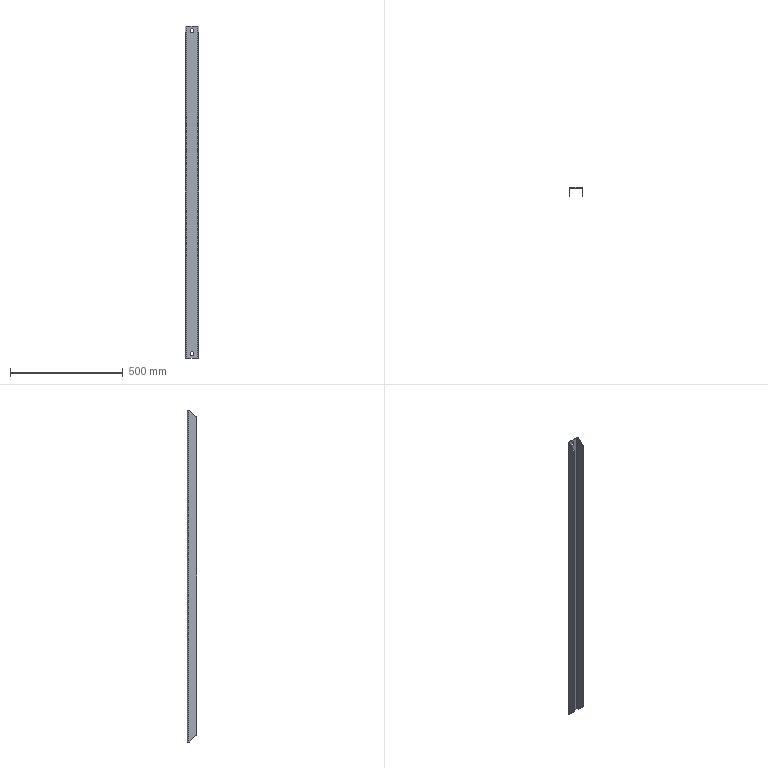Part | STEP file | VD-SYL0380DJ1006_1-2_VD-SYL0380 | 1 solid | 32 faces | box 60 x 40 x 1470 mm | volume 567408 mm3 | plane 18 | cylinder 14 | commonest cylinder face diameters 10 x6 20 x4 6 x2 12 x2
STEP:
#1=CARTESIAN_POINT('',(-5.,20.,-720.));
#2=VERTEX_POINT('',#1);
#3=CARTESIAN_POINT('',(0.,20.,-725.));
#4=VERTEX_POINT('',#3);
#5=CARTESIAN_POINT('',(0.,20.,-720.));
#6=DIRECTION('',(0.,-1.,0.));
#7=DIRECTION('',(-1.,0.,0.));
#8=AXIS2_PLACEMENT_3D('',#5,#6,#7);
#9=CIRCLE('',#8,5.);
#10=EDGE_CURVE('',#2,#4,#9,.T.);
#11=ORIENTED_EDGE('',*,*,#10,.F.);
#12=CARTESIAN_POINT('',(-5.,17.,-720.));
#13=VERTEX_POINT('',#12);
#14=CARTESIAN_POINT('',(-5.,20.,-720.));
#15=DIRECTION('',(0.,-1.,0.));
#16=VECTOR('',#15,1000.);
#17=LINE('',#14,#16);
#18=EDGE_CURVE('',#2,#13,#17,.T.);
#19=ORIENTED_EDGE('',*,*,#18,.T.);
#20=CARTESIAN_POINT('',(0.,17.,-725.));
#21=VERTEX_POINT('',#20);
#22=CARTESIAN_POINT('',(0.,17.,-720.));
#23=DIRECTION('',(0.,1.,0.));
#24=DIRECTION('',(0.,0.,-1.));
#25=AXIS2_PLACEMENT_3D('',#22,#23,#24);
#26=CIRCLE('',#25,5.);
#27=EDGE_CURVE('',#21,#13,#26,.T.);
#28=ORIENTED_EDGE('',*,*,#27,.F.);
#29=CARTESIAN_POINT('',(0.,17.,-725.));
#30=DIRECTION('',(0.,1.,0.));
#31=VECTOR('',#30,1000.);
#32=LINE('',#29,#31);
#33=EDGE_CURVE('',#21,#4,#32,.T.);
#34=ORIENTED_EDGE('',*,*,#33,.T.);
#35=EDGE_LOOP('',(#11,#19,#28,#34));
#36=FACE_OUTER_BOUND('',#35,.T.);
#37=CARTESIAN_POINT('',(0.,18.5,-720.));
#38=DIRECTION('',(0.,-1.,0.));
#39=DIRECTION('',(0.,0.,-1.));
#40=AXIS2_PLACEMENT_3D('',#37,#38,#39);
#41=CYLINDRICAL_SURFACE('',#40,5.);
#42=ADVANCED_FACE('',(#36),#41,.F.);
#43=ORIENTED_EDGE('',*,*,#33,.F.);
#44=CARTESIAN_POINT('',(5.,17.,-720.));
#45=VERTEX_POINT('',#44);
#46=CARTESIAN_POINT('',(0.,17.,-720.));
#47=DIRECTION('',(0.,1.,0.));
#48=DIRECTION('',(1.,0.,0.));
#49=AXIS2_PLACEMENT_3D('',#46,#47,#48);
#50=CIRCLE('',#49,5.);
#51=EDGE_CURVE('',#45,#21,#50,.T.);
#52=ORIENTED_EDGE('',*,*,#51,.F.);
#53=CARTESIAN_POINT('',(5.,20.,-720.));
#54=VERTEX_POINT('',#53);
#55=CARTESIAN_POINT('',(5.,17.,-720.));
#56=DIRECTION('',(0.,1.,0.));
#57=VECTOR('',#56,1000.);
#58=LINE('',#55,#57);
#59=EDGE_CURVE('',#45,#54,#58,.T.);
#60=ORIENTED_EDGE('',*,*,#59,.T.);
#61=CARTESIAN_POINT('',(0.,20.,-720.));
#62=DIRECTION('',(0.,-1.,0.));
#63=DIRECTION('',(0.,0.,-1.));
#64=AXIS2_PLACEMENT_3D('',#61,#62,#63);
#65=CIRCLE('',#64,5.);
#66=EDGE_CURVE('',#4,#54,#65,.T.);
#67=ORIENTED_EDGE('',*,*,#66,.F.);
#68=EDGE_LOOP('',(#43,#52,#60,#67));
#69=FACE_OUTER_BOUND('',#68,.T.);
#70=CARTESIAN_POINT('',(0.,18.5,-720.));
#71=DIRECTION('',(0.,-1.,0.));
#72=DIRECTION('',(0.,0.,-1.));
#73=AXIS2_PLACEMENT_3D('',#70,#71,#72);
#74=CYLINDRICAL_SURFACE('',#73,5.);
#75=ADVANCED_FACE('',(#69),#74,.F.);
#76=CARTESIAN_POINT('',(5.,20.,-710.));
#77=VERTEX_POINT('',#76);
#78=CARTESIAN_POINT('',(5.,17.,-710.));
#79=VERTEX_POINT('',#78);
#80=CARTESIAN_POINT('',(5.,20.,-710.));
#81=DIRECTION('',(0.,-1.,0.));
#82=VECTOR('',#81,1000.);
#83=LINE('',#80,#82);
#84=EDGE_CURVE('',#77,#79,#83,.T.);
#85=ORIENTED_EDGE('',*,*,#84,.F.);
#86=CARTESIAN_POINT('',(5.,20.,-710.));
#87=DIRECTION('',(0.,0.,-1.));
#88=VECTOR('',#87,1000.);
#89=LINE('',#86,#88);
#90=EDGE_CURVE('',#77,#54,#89,.T.);
#91=ORIENTED_EDGE('',*,*,#90,.T.);
#92=ORIENTED_EDGE('',*,*,#59,.F.);
#93=CARTESIAN_POINT('',(5.,17.,-720.));
#94=DIRECTION('',(0.,0.,1.));
#95=VECTOR('',#94,1000.);
#96=LINE('',#93,#95);
#97=EDGE_CURVE('',#45,#79,#96,.T.);
#98=ORIENTED_EDGE('',*,*,#97,.T.);
#99=EDGE_LOOP('',(#85,#91,#92,#98));
#100=FACE_OUTER_BOUND('',#99,.T.);
#101=CARTESIAN_POINT('',(5.,18.5,-717.5));
#102=DIRECTION('',(1.,0.,0.));
#103=DIRECTION('',(0.,1.,0.));
#104=AXIS2_PLACEMENT_3D('',#101,#102,#103);
#105=PLANE('',#104);
#106=ADVANCED_FACE('',(#100),#105,.F.);
#107=CARTESIAN_POINT('',(-5.,17.,-710.));
#108=VERTEX_POINT('',#107);
#109=CARTESIAN_POINT('',(0.,17.,-710.));
#110=DIRECTION('',(0.,1.,0.));
#111=DIRECTION('',(0.,0.,1.));
#112=AXIS2_PLACEMENT_3D('',#109,#110,#111);
#113=CIRCLE('',#112,5.);
#114=EDGE_CURVE('',#108,#79,#113,.T.);
#115=ORIENTED_EDGE('',*,*,#114,.F.);
#116=CARTESIAN_POINT('',(-5.,20.,-710.));
#117=VERTEX_POINT('',#116);
#118=CARTESIAN_POINT('',(-5.,17.,-710.));
#119=DIRECTION('',(0.,1.,0.));
#120=VECTOR('',#119,1000.);
#121=LINE('',#118,#120);
#122=EDGE_CURVE('',#108,#117,#121,.T.);
#123=ORIENTED_EDGE('',*,*,#122,.T.);
#124=CARTESIAN_POINT('',(0.,20.,-710.));
#125=DIRECTION('',(0.,-1.,0.));
#126=DIRECTION('',(1.,0.,0.));
#127=AXIS2_PLACEMENT_3D('',#124,#125,#126);
#128=CIRCLE('',#127,5.);
#129=EDGE_CURVE('',#77,#117,#128,.T.);
#130=ORIENTED_EDGE('',*,*,#129,.F.);
#131=ORIENTED_EDGE('',*,*,#84,.T.);
#132=EDGE_LOOP('',(#115,#123,#130,#131));
#133=FACE_OUTER_BOUND('',#132,.T.);
#134=CARTESIAN_POINT('',(0.,18.5,-710.));
#135=DIRECTION('',(0.,-1.,0.));
#136=DIRECTION('',(0.,0.,-1.));
#137=AXIS2_PLACEMENT_3D('',#134,#135,#136);
#138=CYLINDRICAL_SURFACE('',#137,5.);
#139=ADVANCED_FACE('',(#133),#138,.F.);
#140=CARTESIAN_POINT('',(-5.,20.,710.));
#141=VERTEX_POINT('',#140);
#142=CARTESIAN_POINT('',(-5.,17.,710.));
#143=VERTEX_POINT('',#142);
#144=CARTESIAN_POINT('',(-5.,20.,710.));
#145=DIRECTION('',(0.,-1.,0.));
#146=VECTOR('',#145,1000.);
#147=LINE('',#144,#146);
#148=EDGE_CURVE('',#141,#143,#147,.T.);
#149=ORIENTED_EDGE('',*,*,#148,.F.);
#150=CARTESIAN_POINT('',(-5.,20.,720.));
#151=VERTEX_POINT('',#150);
#152=CARTESIAN_POINT('',(-5.,20.,710.));
#153=DIRECTION('',(0.,0.,1.));
#154=VECTOR('',#153,1000.);
#155=LINE('',#152,#154);
#156=EDGE_CURVE('',#141,#151,#155,.T.);
#157=ORIENTED_EDGE('',*,*,#156,.T.);
#158=CARTESIAN_POINT('',(-5.,17.,720.));
#159=VERTEX_POINT('',#158);
#160=CARTESIAN_POINT('',(-5.,17.,720.));
#161=DIRECTION('',(0.,1.,0.));
#162=VECTOR('',#161,1000.);
#163=LINE('',#160,#162);
#164=EDGE_CURVE('',#159,#151,#163,.T.);
#165=ORIENTED_EDGE('',*,*,#164,.F.);
#166=CARTESIAN_POINT('',(-5.,17.,720.));
#167=DIRECTION('',(0.,0.,-1.));
#168=VECTOR('',#167,1000.);
#169=LINE('',#166,#168);
#170=EDGE_CURVE('',#159,#143,#169,.T.);
#171=ORIENTED_EDGE('',*,*,#170,.T.);
#172=EDGE_LOOP('',(#149,#157,#165,#171));
#173=FACE_OUTER_BOUND('',#172,.T.);
#174=CARTESIAN_POINT('',(-5.,18.5,717.5));
#175=DIRECTION('',(-1.,0.,0.));
#176=DIRECTION('',(0.,0.,1.));
#177=AXIS2_PLACEMENT_3D('',#174,#175,#176);
#178=PLANE('',#177);
#179=ADVANCED_FACE('',(#173),#178,.F.);
#180=CARTESIAN_POINT('',(5.,17.,720.));
#181=VERTEX_POINT('',#180);
#182=CARTESIAN_POINT('',(0.,17.,720.));
#183=DIRECTION('',(0.,1.,0.));
#184=DIRECTION('',(-1.,0.,0.));
#185=AXIS2_PLACEMENT_3D('',#182,#183,#184);
#186=CIRCLE('',#185,5.);
#187=EDGE_CURVE('',#159,#181,#186,.T.);
#188=ORIENTED_EDGE('',*,*,#187,.F.);
#189=ORIENTED_EDGE('',*,*,#164,.T.);
#190=CARTESIAN_POINT('',(5.,20.,720.));
#191=VERTEX_POINT('',#190);
#192=CARTESIAN_POINT('',(0.,20.,720.));
#193=DIRECTION('',(0.,-1.,0.));
#194=DIRECTION('',(1.,0.,0.));
#195=AXIS2_PLACEMENT_3D('',#192,#193,#194);
#196=CIRCLE('',#195,5.);
#197=EDGE_CURVE('',#191,#151,#196,.T.);
#198=ORIENTED_EDGE('',*,*,#197,.F.);
#199=CARTESIAN_POINT('',(5.,20.,720.));
#200=DIRECTION('',(0.,-1.,0.));
#201=VECTOR('',#200,1000.);
#202=LINE('',#199,#201);
#203=EDGE_CURVE('',#191,#181,#202,.T.);
#204=ORIENTED_EDGE('',*,*,#203,.T.);
#205=EDGE_LOOP('',(#188,#189,#198,#204));
#206=FACE_OUTER_BOUND('',#205,.T.);
#207=CARTESIAN_POINT('',(0.,18.5,720.));
#208=DIRECTION('',(0.,-1.,0.));
#209=DIRECTION('',(0.,0.,-1.));
#210=AXIS2_PLACEMENT_3D('',#207,#208,#209);
#211=CYLINDRICAL_SURFACE('',#210,5.);
#212=ADVANCED_FACE('',(#206),#211,.F.);
#213=ORIENTED_EDGE('',*,*,#203,.F.);
#214=CARTESIAN_POINT('',(5.,20.,710.));
#215=VERTEX_POINT('',#214);
#216=CARTESIAN_POINT('',(5.,20.,720.));
#217=DIRECTION('',(0.,0.,-1.));
#218=VECTOR('',#217,1000.);
#219=LINE('',#216,#218);
#220=EDGE_CURVE('',#191,#215,#219,.T.);
#221=ORIENTED_EDGE('',*,*,#220,.T.);
#222=CARTESIAN_POINT('',(5.,17.,710.));
#223=VERTEX_POINT('',#222);
#224=CARTESIAN_POINT('',(5.,17.,710.));
#225=DIRECTION('',(0.,1.,0.));
#226=VECTOR('',#225,1000.);
#227=LINE('',#224,#226);
#228=EDGE_CURVE('',#223,#215,#227,.T.);
#229=ORIENTED_EDGE('',*,*,#228,.F.);
#230=CARTESIAN_POINT('',(5.,17.,710.));
#231=DIRECTION('',(0.,0.,1.));
#232=VECTOR('',#231,1000.);
#233=LINE('',#230,#232);
#234=EDGE_CURVE('',#223,#181,#233,.T.);
#235=ORIENTED_EDGE('',*,*,#234,.T.);
#236=EDGE_LOOP('',(#213,#221,#229,#235));
#237=FACE_OUTER_BOUND('',#236,.T.);
#238=CARTESIAN_POINT('',(5.,18.5,712.5));
#239=DIRECTION('',(1.,0.,0.));
#240=DIRECTION('',(0.,1.,0.));
#241=AXIS2_PLACEMENT_3D('',#238,#239,#240);
#242=PLANE('',#241);
#243=ADVANCED_FACE('',(#237),#242,.F.);
#244=CARTESIAN_POINT('',(0.,17.,705.));
#245=VERTEX_POINT('',#244);
#246=CARTESIAN_POINT('',(0.,20.,705.));
#247=VERTEX_POINT('',#246);
#248=CARTESIAN_POINT('',(0.,17.,705.));
#249=DIRECTION('',(0.,1.,0.));
#250=VECTOR('',#249,1000.);
#251=LINE('',#248,#250);
#252=EDGE_CURVE('',#245,#247,#251,.T.);
#253=ORIENTED_EDGE('',*,*,#252,.F.);
#254=CARTESIAN_POINT('',(0.,17.,710.));
#255=DIRECTION('',(0.,1.,0.));
#256=DIRECTION('',(1.,0.,0.));
#257=AXIS2_PLACEMENT_3D('',#254,#255,#256);
#258=CIRCLE('',#257,5.);
#259=EDGE_CURVE('',#223,#245,#258,.T.);
#260=ORIENTED_EDGE('',*,*,#259,.F.);
#261=ORIENTED_EDGE('',*,*,#228,.T.);
#262=CARTESIAN_POINT('',(0.,20.,710.));
#263=DIRECTION('',(0.,-1.,0.));
#264=DIRECTION('',(0.,0.,-1.));
#265=AXIS2_PLACEMENT_3D('',#262,#263,#264);
#266=CIRCLE('',#265,5.);
#267=EDGE_CURVE('',#247,#215,#266,.T.);
#268=ORIENTED_EDGE('',*,*,#267,.F.);
#269=EDGE_LOOP('',(#253,#260,#261,#268));
#270=FACE_OUTER_BOUND('',#269,.T.);
#271=CARTESIAN_POINT('',(0.,18.5,710.));
#272=DIRECTION('',(0.,-1.,0.));
#273=DIRECTION('',(0.,0.,-1.));
#274=AXIS2_PLACEMENT_3D('',#271,#272,#273);
#275=CYLINDRICAL_SURFACE('',#274,5.);
#276=ADVANCED_FACE('',(#270),#275,.F.);
#277=CARTESIAN_POINT('',(0.,20.,710.));
#278=DIRECTION('',(0.,-1.,0.));
#279=DIRECTION('',(-1.,0.,0.));
#280=AXIS2_PLACEMENT_3D('',#277,#278,#279);
#281=CIRCLE('',#280,5.);
#282=EDGE_CURVE('',#141,#247,#281,.T.);
#283=ORIENTED_EDGE('',*,*,#282,.F.);
#284=ORIENTED_EDGE('',*,*,#148,.T.);
#285=CARTESIAN_POINT('',(0.,17.,710.));
#286=DIRECTION('',(0.,1.,0.));
#287=DIRECTION('',(0.,0.,-1.));
#288=AXIS2_PLACEMENT_3D('',#285,#286,#287);
#289=CIRCLE('',#288,5.);
#290=EDGE_CURVE('',#245,#143,#289,.T.);
#291=ORIENTED_EDGE('',*,*,#290,.F.);
#292=ORIENTED_EDGE('',*,*,#252,.T.);
#293=EDGE_LOOP('',(#283,#284,#291,#292));
#294=FACE_OUTER_BOUND('',#293,.T.);
#295=CARTESIAN_POINT('',(0.,18.5,710.));
#296=DIRECTION('',(0.,-1.,0.));
#297=DIRECTION('',(0.,0.,-1.));
#298=AXIS2_PLACEMENT_3D('',#295,#296,#297);
#299=CYLINDRICAL_SURFACE('',#298,5.);
#300=ADVANCED_FACE('',(#294),#299,.F.);
#301=CARTESIAN_POINT('',(-24.,17.,-735.));
#302=VERTEX_POINT('',#301);
#303=CARTESIAN_POINT('',(-27.,14.,-735.));
#304=VERTEX_POINT('',#303);
#305=CARTESIAN_POINT('',(-24.,14.,-735.));
#306=DIRECTION('',(0.,0.,1.));
#307=DIRECTION('',(0.,1.,0.));
#308=AXIS2_PLACEMENT_3D('',#305,#306,#307);
#309=CIRCLE('',#308,3.);
#310=EDGE_CURVE('',#302,#304,#309,.T.);
#311=ORIENTED_EDGE('',*,*,#310,.F.);
#312=CARTESIAN_POINT('',(-24.,17.,735.));
#313=VERTEX_POINT('',#312);
#314=CARTESIAN_POINT('',(-24.,17.,-735.));
#315=DIRECTION('',(0.,0.,1.));
#316=VECTOR('',#315,1000.);
#317=LINE('',#314,#316);
#318=EDGE_CURVE('',#302,#313,#317,.T.);
#319=ORIENTED_EDGE('',*,*,#318,.T.);
#320=CARTESIAN_POINT('',(-27.,14.,735.));
#321=VERTEX_POINT('',#320);
#322=CARTESIAN_POINT('',(-24.,14.,735.));
#323=DIRECTION('',(0.,0.,-1.));
#324=DIRECTION('',(-1.,0.,0.));
#325=AXIS2_PLACEMENT_3D('',#322,#323,#324);
#326=CIRCLE('',#325,3.);
#327=EDGE_CURVE('',#321,#313,#326,.T.);
#328=ORIENTED_EDGE('',*,*,#327,.F.);
#329=CARTESIAN_POINT('',(-27.,14.,735.));
#330=DIRECTION('',(0.,0.,-1.));
#331=VECTOR('',#330,1000.);
#332=LINE('',#329,#331);
#333=EDGE_CURVE('',#321,#304,#332,.T.);
#334=ORIENTED_EDGE('',*,*,#333,.T.);
#335=EDGE_LOOP('',(#311,#319,#328,#334));
#336=FACE_OUTER_BOUND('',#335,.T.);
#337=CARTESIAN_POINT('',(-24.,14.,2651.292));
#338=DIRECTION('',(0.,0.,-1.));
#339=DIRECTION('',(-1.,0.,0.));
#340=AXIS2_PLACEMENT_3D('',#337,#338,#339);
#341=CYLINDRICAL_SURFACE('',#340,3.);
#342=ADVANCED_FACE('',(#336),#341,.F.);
#343=CARTESIAN_POINT('',(-27.,-17.071,707.929));
#344=VERTEX_POINT('',#343);
#345=CARTESIAN_POINT('',(-30.,-17.071,707.929));
#346=VERTEX_POINT('',#345);
#347=CARTESIAN_POINT('',(-27.,-17.071,707.929));
#348=DIRECTION('',(-1.,0.,0.));
#349=VECTOR('',#348,1000.);
#350=LINE('',#347,#349);
#351=EDGE_CURVE('',#344,#346,#350,.T.);
#352=ORIENTED_EDGE('',*,*,#351,.F.);
#353=CARTESIAN_POINT('',(-27.,10.,735.));
#354=VERTEX_POINT('',#353);
#355=CARTESIAN_POINT('',(-27.,10.,735.));
#356=DIRECTION('',(0.,-0.7071,-0.7071));
#357=VECTOR('',#356,1000.);
#358=LINE('',#355,#357);
#359=EDGE_CURVE('',#354,#344,#358,.T.);
#360=ORIENTED_EDGE('',*,*,#359,.F.);
#361=CARTESIAN_POINT('',(-30.,10.,735.));
#362=VERTEX_POINT('',#361);
#363=CARTESIAN_POINT('',(-30.,10.,735.));
#364=DIRECTION('',(1.,0.,0.));
#365=VECTOR('',#364,1000.);
#366=LINE('',#363,#365);
#367=EDGE_CURVE('',#362,#354,#366,.T.);
#368=ORIENTED_EDGE('',*,*,#367,.F.);
#369=CARTESIAN_POINT('',(-30.,-17.071,707.929));
#370=DIRECTION('',(0.,0.7071,0.7071));
#371=VECTOR('',#370,1000.);
#372=LINE('',#369,#371);
#373=EDGE_CURVE('',#346,#362,#372,.T.);
#374=ORIENTED_EDGE('',*,*,#373,.F.);
#375=EDGE_LOOP('',(#352,#360,#368,#374));
#376=FACE_OUTER_BOUND('',#375,.T.);
#377=CARTESIAN_POINT('',(-28.5,-5.,720.));
#378=DIRECTION('',(0.,-0.7071,0.7071));
#379=DIRECTION('',(-1.,0.,0.));
#380=AXIS2_PLACEMENT_3D('',#377,#378,#379);
#381=PLANE('',#380);
#382=ADVANCED_FACE('',(#376),#381,.T.);
#383=CARTESIAN_POINT('',(-30.,-20.,700.858));
#384=VERTEX_POINT('',#383);
#385=CARTESIAN_POINT('',(-30.,-10.,700.858));
#386=DIRECTION('',(-1.,0.,0.));
#387=DIRECTION('',(0.,-1.,0.));
#388=AXIS2_PLACEMENT_3D('',#385,#386,#387);
#389=CIRCLE('',#388,10.);
#390=EDGE_CURVE('',#384,#346,#389,.T.);
#391=ORIENTED_EDGE('',*,*,#390,.F.);
#392=CARTESIAN_POINT('',(-27.,-20.,700.858));
#393=VERTEX_POINT('',#392);
#394=CARTESIAN_POINT('',(-30.,-20.,700.858));
#395=DIRECTION('',(1.,0.,0.));
#396=VECTOR('',#395,1000.);
#397=LINE('',#394,#396);
#398=EDGE_CURVE('',#384,#393,#397,.T.);
#399=ORIENTED_EDGE('',*,*,#398,.T.);
#400=CARTESIAN_POINT('',(-27.,-10.,700.858));
#401=DIRECTION('',(1.,0.,0.));
#402=DIRECTION('',(0.,-0.7071,0.7071));
#403=AXIS2_PLACEMENT_3D('',#400,#401,#402);
#404=CIRCLE('',#403,10.);
#405=EDGE_CURVE('',#344,#393,#404,.T.);
#406=ORIENTED_EDGE('',*,*,#405,.F.);
#407=ORIENTED_EDGE('',*,*,#351,.T.);
#408=EDGE_LOOP('',(#391,#399,#406,#407));
#409=FACE_OUTER_BOUND('',#408,.T.);
#410=CARTESIAN_POINT('',(108.216,-10.,700.858));
#411=DIRECTION('',(-1.,0.,0.));
#412=DIRECTION('',(0.,0.,1.));
#413=AXIS2_PLACEMENT_3D('',#410,#411,#412);
#414=CYLINDRICAL_SURFACE('',#413,10.);
#415=ADVANCED_FACE('',(#409),#414,.T.);
#416=CARTESIAN_POINT('',(-30.,-17.071,-707.929));
#417=VERTEX_POINT('',#416);
#418=CARTESIAN_POINT('',(-27.,-17.071,-707.929));
#419=VERTEX_POINT('',#418);
#420=CARTESIAN_POINT('',(-30.,-17.071,-707.929));
#421=DIRECTION('',(1.,0.,0.));
#422=VECTOR('',#421,1000.);
#423=LINE('',#420,#422);
#424=EDGE_CURVE('',#417,#419,#423,.T.);
#425=ORIENTED_EDGE('',*,*,#424,.F.);
#426=CARTESIAN_POINT('',(-30.,10.,-735.));
#427=VERTEX_POINT('',#426);
#428=CARTESIAN_POINT('',(-30.,10.,-735.));
#429=DIRECTION('',(0.,-0.7071,0.7071));
#430=VECTOR('',#429,1000.);
#431=LINE('',#428,#430);
#432=EDGE_CURVE('',#427,#417,#431,.T.);
#433=ORIENTED_EDGE('',*,*,#432,.F.);
#434=CARTESIAN_POINT('',(-27.,10.,-735.));
#435=VERTEX_POINT('',#434);
#436=CARTESIAN_POINT('',(-27.,10.,-735.));
#437=DIRECTION('',(-1.,0.,0.));
#438=VECTOR('',#437,1000.);
#439=LINE('',#436,#438);
#440=EDGE_CURVE('',#435,#427,#439,.T.);
#441=ORIENTED_EDGE('',*,*,#440,.F.);
#442=CARTESIAN_POINT('',(-27.,-17.071,-707.929));
#443=DIRECTION('',(0.,0.7071,-0.7071));
#444=VECTOR('',#443,1000.);
#445=LINE('',#442,#444);
#446=EDGE_CURVE('',#419,#435,#445,.T.);
#447=ORIENTED_EDGE('',*,*,#446,.F.);
#448=EDGE_LOOP('',(#425,#433,#441,#447));
#449=FACE_OUTER_BOUND('',#448,.T.);
#450=CARTESIAN_POINT('',(-28.5,-5.,-720.));
#451=DIRECTION('',(0.,-0.7071,-0.7071));
#452=DIRECTION('',(0.,-0.7071,0.7071));
#453=AXIS2_PLACEMENT_3D('',#450,#451,#452);
#454=PLANE('',#453);
#455=ADVANCED_FACE('',(#449),#454,.T.);
#456=CARTESIAN_POINT('',(-27.,-20.,-700.858));
#457=VERTEX_POINT('',#456);
#458=CARTESIAN_POINT('',(-27.,-10.,-700.858));
#459=DIRECTION('',(1.,0.,0.));
#460=DIRECTION('',(0.,-1.,0.));
#461=AXIS2_PLACEMENT_3D('',#458,#459,#460);
#462=CIRCLE('',#461,10.);
#463=EDGE_CURVE('',#457,#419,#462,.T.);
#464=ORIENTED_EDGE('',*,*,#463,.F.);
#465=CARTESIAN_POINT('',(-30.,-20.,-700.858));
#466=VERTEX_POINT('',#465);
#467=CARTESIAN_POINT('',(-27.,-20.,-700.858));
#468=DIRECTION('',(-1.,0.,0.));
#469=VECTOR('',#468,1000.);
#470=LINE('',#467,#469);
#471=EDGE_CURVE('',#457,#466,#470,.T.);
#472=ORIENTED_EDGE('',*,*,#471,.T.);
#473=CARTESIAN_POINT('',(-30.,-10.,-700.858));
#474=DIRECTION('',(-1.,0.,0.));
#475=DIRECTION('',(0.,-0.7071,-0.7071));
#476=AXIS2_PLACEMENT_3D('',#473,#474,#475);
#477=CIRCLE('',#476,10.);
#478=EDGE_CURVE('',#417,#466,#477,.T.);
#479=ORIENTED_EDGE('',*,*,#478,.F.);
#480=ORIENTED_EDGE('',*,*,#424,.T.);
#481=EDGE_LOOP('',(#464,#472,#479,#480));
#482=FACE_OUTER_BOUND('',#481,.T.);
#483=CARTESIAN_POINT('',(-108.216,-10.,-700.858));
#484=DIRECTION('',(1.,0.,0.));
#485=DIRECTION('',(0.,0.,-1.));
#486=AXIS2_PLACEMENT_3D('',#483,#484,#485);
#487=CYLINDRICAL_SURFACE('',#486,10.);
#488=ADVANCED_FACE('',(#482),#487,.T.);
#489=ORIENTED_EDGE('',*,*,#446,.T.);
#490=CARTESIAN_POINT('',(-27.,10.,-735.));
#491=DIRECTION('',(0.,1.,0.));
#492=VECTOR('',#491,1000.);
#493=LINE('',#490,#492);
#494=EDGE_CURVE('',#435,#304,#493,.T.);
#495=ORIENTED_EDGE('',*,*,#494,.T.);
#496=ORIENTED_EDGE('',*,*,#333,.F.);
#497=CARTESIAN_POINT('',(-27.,10.,735.));
#498=DIRECTION('',(0.,1.,0.));
#499=VECTOR('',#498,1000.);
#500=LINE('',#497,#499);
#501=EDGE_CURVE('',#354,#321,#500,.T.);
#502=ORIENTED_EDGE('',*,*,#501,.F.);
#503=ORIENTED_EDGE('',*,*,#359,.T.);
#504=ORIENTED_EDGE('',*,*,#405,.T.);
#505=CARTESIAN_POINT('',(-27.,-20.,700.858));
#506=DIRECTION('',(0.,0.,-1.));
#507=VECTOR('',#506,1000.);
#508=LINE('',#505,#507);
#509=EDGE_CURVE('',#393,#457,#508,.T.);
#510=ORIENTED_EDGE('',*,*,#509,.T.);
#511=ORIENTED_EDGE('',*,*,#463,.T.);
#512=EDGE_LOOP('',(#489,#495,#496,#502,#503,#504,#510,#511));
#513=FACE_OUTER_BOUND('',#512,.T.);
#514=CARTESIAN_POINT('',(-27.,20.,-735.));
#515=DIRECTION('',(-1.,0.,0.));
#516=DIRECTION('',(0.,0.,1.));
#517=AXIS2_PLACEMENT_3D('',#514,#515,#516);
#518=PLANE('',#517);
#519=ADVANCED_FACE('',(#513),#518,.F.);
#520=ORIENTED_EDGE('',*,*,#398,.F.);
#521=CARTESIAN_POINT('',(-30.,-20.,700.858));
#522=DIRECTION('',(0.,0.,-1.));
#523=VECTOR('',#522,1000.);
#524=LINE('',#521,#523);
#525=EDGE_CURVE('',#384,#466,#524,.T.);
#526=ORIENTED_EDGE('',*,*,#525,.T.);
#527=ORIENTED_EDGE('',*,*,#471,.F.);
#528=ORIENTED_EDGE('',*,*,#509,.F.);
#529=EDGE_LOOP('',(#520,#526,#527,#528));
#530=FACE_OUTER_BOUND('',#529,.T.);
#531=CARTESIAN_POINT('',(-28.5,-20.,0.));
#532=DIRECTION('',(0.,-1.,0.));
#533=DIRECTION('',(0.,0.,-1.));
#534=AXIS2_PLACEMENT_3D('',#531,#532,#533);
#535=PLANE('',#534);
#536=ADVANCED_FACE('',(#530),#535,.T.);
#537=ORIENTED_EDGE('',*,*,#390,.T.);
#538=ORIENTED_EDGE('',*,*,#373,.T.);
#539=CARTESIAN_POINT('',(-30.,14.,735.));
#540=VERTEX_POINT('',#539);
#541=CARTESIAN_POINT('',(-30.,14.,735.));
#542=DIRECTION('',(0.,-1.,0.));
#543=VECTOR('',#542,1000.);
#544=LINE('',#541,#543);
#545=EDGE_CURVE('',#540,#362,#544,.T.);
#546=ORIENTED_EDGE('',*,*,#545,.F.);
#547=CARTESIAN_POINT('',(-30.,14.,-735.));
#548=VERTEX_POINT('',#547);
#549=CARTESIAN_POINT('',(-30.,14.,-735.));
#550=DIRECTION('',(0.,0.,1.));
#551=VECTOR('',#550,1000.);
#552=LINE('',#549,#551);
#553=EDGE_CURVE('',#548,#540,#552,.T.);
#554=ORIENTED_EDGE('',*,*,#553,.F.);
#555=CARTESIAN_POINT('',(-30.,10.,-735.));
#556=DIRECTION('',(0.,1.,0.));
#557=VECTOR('',#556,1000.);
#558=LINE('',#555,#557);
#559=EDGE_CURVE('',#427,#548,#558,.T.);
#560=ORIENTED_EDGE('',*,*,#559,.F.);
#561=ORIENTED_EDGE('',*,*,#432,.T.);
#562=ORIENTED_EDGE('',*,*,#478,.T.);
#563=ORIENTED_EDGE('',*,*,#525,.F.);
#564=EDGE_LOOP('',(#537,#538,#546,#554,#560,#561,#562,#563));
#565=FACE_OUTER_BOUND('',#564,.T.);
#566=CARTESIAN_POINT('',(-30.,20.,-735.));
#567=DIRECTION('',(-1.,0.,0.));
#568=DIRECTION('',(0.,0.,1.));
#569=AXIS2_PLACEMENT_3D('',#566,#567,#568);
#570=PLANE('',#569);
#571=ADVANCED_FACE('',(#565),#570,.T.);
#572=CARTESIAN_POINT('',(-24.,20.,735.));
#573=VERTEX_POINT('',#572);
#574=CARTESIAN_POINT('',(-24.,20.,-735.));
#575=VERTEX_POINT('',#574);
#576=CARTESIAN_POINT('',(-24.,20.,735.));
#577=DIRECTION('',(0.,0.,-1.));
#578=VECTOR('',#577,1000.);
#579=LINE('',#576,#578);
#580=EDGE_CURVE('',#573,#575,#579,.T.);
#581=ORIENTED_EDGE('',*,*,#580,.T.);
#582=CARTESIAN_POINT('',(-24.,14.,-735.));
#583=DIRECTION('',(0.,0.,-1.));
#584=DIRECTION('',(-1.,0.,0.));
#585=AXIS2_PLACEMENT_3D('',#582,#583,#584);
#586=CIRCLE('',#585,6.);
#587=EDGE_CURVE('',#548,#575,#586,.T.);
#588=ORIENTED_EDGE('',*,*,#587,.F.);
#589=ORIENTED_EDGE('',*,*,#553,.T.);
#590=CARTESIAN_POINT('',(-24.,14.,735.));
#591=DIRECTION('',(0.,0.,1.));
#592=DIRECTION('',(0.,1.,0.));
#593=AXIS2_PLACEMENT_3D('',#590,#591,#592);
#594=CIRCLE('',#593,6.);
#595=EDGE_CURVE('',#573,#540,#594,.T.);
#596=ORIENTED_EDGE('',*,*,#595,.F.);
#597=EDGE_LOOP('',(#581,#588,#589,#596));
#598=FACE_OUTER_BOUND('',#597,.T.);
#599=CARTESIAN_POINT('',(-24.,14.,2651.292));
#600=DIRECTION('',(0.,0.,-1.));
#601=DIRECTION('',(-1.,0.,0.));
#602=AXIS2_PLACEMENT_3D('',#599,#600,#601);
#603=CYLINDRICAL_SURFACE('',#602,6.);
#604=ADVANCED_FACE('',(#598),#603,.T.);
#605=CARTESIAN_POINT('',(27.,-20.,700.858));
#606=VERTEX_POINT('',#605);
#607=CARTESIAN_POINT('',(27.,-17.071,707.929));
#608=VERTEX_POINT('',#607);
#609=CARTESIAN_POINT('',(27.,-10.,700.858));
#610=DIRECTION('',(-1.,0.,0.));
#611=DIRECTION('',(0.,-1.,0.));
#612=AXIS2_PLACEMENT_3D('',#609,#610,#611);
#613=CIRCLE('',#612,10.);
#614=EDGE_CURVE('',#606,#608,#613,.T.);
#615=ORIENTED_EDGE('',*,*,#614,.F.);
#616=CARTESIAN_POINT('',(30.,-20.,700.858));
#617=VERTEX_POINT('',#616);
#618=CARTESIAN_POINT('',(27.,-20.,700.858));
#619=DIRECTION('',(1.,0.,0.));
#620=VECTOR('',#619,1000.);
#621=LINE('',#618,#620);
#622=EDGE_CURVE('',#606,#617,#621,.T.);
#623=ORIENTED_EDGE('',*,*,#622,.T.);
#624=CARTESIAN_POINT('',(30.,-17.071,707.929));
#625=VERTEX_POINT('',#624);
#626=CARTESIAN_POINT('',(30.,-10.,700.858));
#627=DIRECTION('',(1.,0.,0.));
#628=DIRECTION('',(0.,-0.7071,0.7071));
#629=AXIS2_PLACEMENT_3D('',#626,#627,#628);
#630=CIRCLE('',#629,10.);
#631=EDGE_CURVE('',#625,#617,#630,.T.);
#632=ORIENTED_EDGE('',*,*,#631,.F.);
#633=CARTESIAN_POINT('',(30.,-17.071,707.929));
#634=DIRECTION('',(-1.,0.,0.));
#635=VECTOR('',#634,1000.);
#636=LINE('',#633,#635);
#637=EDGE_CURVE('',#625,#608,#636,.T.);
#638=ORIENTED_EDGE('',*,*,#637,.T.);
#639=EDGE_LOOP('',(#615,#623,#632,#638));
#640=FACE_OUTER_BOUND('',#639,.T.);
#641=CARTESIAN_POINT('',(108.216,-10.,700.858));
#642=DIRECTION('',(-1.,0.,0.));
#643=DIRECTION('',(0.,0.,1.));
#644=AXIS2_PLACEMENT_3D('',#641,#642,#643);
#645=CYLINDRICAL_SURFACE('',#644,10.);
#646=ADVANCED_FACE('',(#640),#645,.T.);
#647=CARTESIAN_POINT('',(30.,-20.,-700.858));
#648=VERTEX_POINT('',#647);
#649=CARTESIAN_POINT('',(30.,-20.,-700.858));
#650=DIRECTION('',(0.,0.,1.));
#651=VECTOR('',#650,1000.);
#652=LINE('',#649,#651);
#653=EDGE_CURVE('',#648,#617,#652,.T.);
#654=ORIENTED_EDGE('',*,*,#653,.T.);
#655=ORIENTED_EDGE('',*,*,#622,.F.);
#656=CARTESIAN_POINT('',(27.,-20.,-700.858));
#657=VERTEX_POINT('',#656);
#658=CARTESIAN_POINT('',(27.,-20.,700.858));
#659=DIRECTION('',(0.,0.,-1.));
#660=VECTOR('',#659,1000.);
#661=LINE('',#658,#660);
#662=EDGE_CURVE('',#606,#657,#661,.T.);
#663=ORIENTED_EDGE('',*,*,#662,.T.);
#664=CARTESIAN_POINT('',(30.,-20.,-700.858));
#665=DIRECTION('',(-1.,0.,0.));
#666=VECTOR('',#665,1000.);
#667=LINE('',#664,#666);
#668=EDGE_CURVE('',#648,#657,#667,.T.);
#669=ORIENTED_EDGE('',*,*,#668,.F.);
#670=EDGE_LOOP('',(#654,#655,#663,#669));
#671=FACE_OUTER_BOUND('',#670,.T.);
#672=CARTESIAN_POINT('',(28.5,-20.,0.));
#673=DIRECTION('',(0.,1.,0.));
#674=DIRECTION('',(1.,0.,0.));
#675=AXIS2_PLACEMENT_3D('',#672,#673,#674);
#676=PLANE('',#675);
#677=ADVANCED_FACE('',(#671),#676,.F.);
#678=CARTESIAN_POINT('',(30.,-17.071,-707.929));
#679=VERTEX_POINT('',#678);
#680=CARTESIAN_POINT('',(30.,-10.,-700.858));
#681=DIRECTION('',(1.,0.,0.));
#682=DIRECTION('',(0.,-1.,0.));
#683=AXIS2_PLACEMENT_3D('',#680,#681,#682);
#684=CIRCLE('',#683,10.);
#685=EDGE_CURVE('',#648,#679,#684,.T.);
#686=ORIENTED_EDGE('',*,*,#685,.F.);
#687=ORIENTED_EDGE('',*,*,#668,.T.);
#688=CARTESIAN_POINT('',(27.,-17.071,-707.929));
#689=VERTEX_POINT('',#688);
#690=CARTESIAN_POINT('',(27.,-10.,-700.858));
#691=DIRECTION('',(-1.,0.,0.));
#692=DIRECTION('',(0.,-0.7071,-0.7071));
#693=AXIS2_PLACEMENT_3D('',#690,#691,#692);
#694=CIRCLE('',#693,10.);
#695=EDGE_CURVE('',#689,#657,#694,.T.);
#696=ORIENTED_EDGE('',*,*,#695,.F.);
#697=CARTESIAN_POINT('',(27.,-17.071,-707.929));
#698=DIRECTION('',(1.,0.,0.));
#699=VECTOR('',#698,1000.);
#700=LINE('',#697,#699);
#701=EDGE_CURVE('',#689,#679,#700,.T.);
#702=ORIENTED_EDGE('',*,*,#701,.T.);
#703=EDGE_LOOP('',(#686,#687,#696,#702));
#704=FACE_OUTER_BOUND('',#703,.T.);
#705=CARTESIAN_POINT('',(-108.216,-10.,-700.858));
#706=DIRECTION('',(1.,0.,0.));
#707=DIRECTION('',(0.,0.,-1.));
#708=AXIS2_PLACEMENT_3D('',#705,#706,#707);
#709=CYLINDRICAL_SURFACE('',#708,10.);
#710=ADVANCED_FACE('',(#704),#709,.T.);
#711=ORIENTED_EDGE('',*,*,#701,.F.);
#712=CARTESIAN_POINT('',(27.,10.,-735.));
#713=VERTEX_POINT('',#712);
#714=CARTESIAN_POINT('',(27.,10.,-735.));
#715=DIRECTION('',(0.,-0.7071,0.7071));
#716=VECTOR('',#715,1000.);
#717=LINE('',#714,#716);
#718=EDGE_CURVE('',#713,#689,#717,.T.);
#719=ORIENTED_EDGE('',*,*,#718,.F.);
#720=CARTESIAN_POINT('',(30.,10.,-735.));
#721=VERTEX_POINT('',#720);
#722=CARTESIAN_POINT('',(27.,10.,-735.));
#723=DIRECTION('',(1.,0.,0.));
#724=VECTOR('',#723,1000.);
#725=LINE('',#722,#724);
#726=EDGE_CURVE('',#713,#721,#725,.T.);
#727=ORIENTED_EDGE('',*,*,#726,.T.);
#728=CARTESIAN_POINT('',(30.,-17.071,-707.929));
#729=DIRECTION('',(0.,0.7071,-0.7071));
#730=VECTOR('',#729,1000.);
#731=LINE('',#728,#730);
#732=EDGE_CURVE('',#679,#721,#731,.T.);
#733=ORIENTED_EDGE('',*,*,#732,.F.);
#734=EDGE_LOOP('',(#711,#719,#727,#733));
#735=FACE_OUTER_BOUND('',#734,.T.);
#736=CARTESIAN_POINT('',(28.5,-5.,-720.));
#737=DIRECTION('',(0.,-0.7071,-0.7071));
#738=DIRECTION('',(0.,-0.7071,0.7071));
#739=AXIS2_PLACEMENT_3D('',#736,#737,#738);
#740=PLANE('',#739);
#741=ADVANCED_FACE('',(#735),#740,.T.);
#742=CARTESIAN_POINT('',(30.,14.,735.));
#743=VERTEX_POINT('',#742);
#744=CARTESIAN_POINT('',(30.,14.,-735.));
#745=VERTEX_POINT('',#744);
#746=CARTESIAN_POINT('',(30.,14.,735.));
#747=DIRECTION('',(0.,0.,-1.));
#748=VECTOR('',#747,1000.);
#749=LINE('',#746,#748);
#750=EDGE_CURVE('',#743,#745,#749,.T.);
#751=ORIENTED_EDGE('',*,*,#750,.T.);
#752=CARTESIAN_POINT('',(24.,20.,-735.));
#753=VERTEX_POINT('',#752);
#754=CARTESIAN_POINT('',(24.,14.,-735.));
#755=DIRECTION('',(0.,0.,-1.));
#756=DIRECTION('',(0.,1.,0.));
#757=AXIS2_PLACEMENT_3D('',#754,#755,#756);
#758=CIRCLE('',#757,6.);
#759=EDGE_CURVE('',#753,#745,#758,.T.);
#760=ORIENTED_EDGE('',*,*,#759,.F.);
#761=CARTESIAN_POINT('',(24.,20.,735.));
#762=VERTEX_POINT('',#761);
#763=CARTESIAN_POINT('',(24.,20.,-735.));
#764=DIRECTION('',(0.,0.,1.));
#765=VECTOR('',#764,1000.);
#766=LINE('',#763,#765);
#767=EDGE_CURVE('',#753,#762,#766,.T.);
#768=ORIENTED_EDGE('',*,*,#767,.T.);
#769=CARTESIAN_POINT('',(24.,14.,735.));
#770=DIRECTION('',(0.,0.,1.));
#771=DIRECTION('',(1.,0.,0.));
#772=AXIS2_PLACEMENT_3D('',#769,#770,#771);
#773=CIRCLE('',#772,6.);
#774=EDGE_CURVE('',#743,#762,#773,.T.);
#775=ORIENTED_EDGE('',*,*,#774,.F.);
#776=EDGE_LOOP('',(#751,#760,#768,#775));
#777=FACE_OUTER_BOUND('',#776,.T.);
#778=CARTESIAN_POINT('',(24.,14.,2651.292));
#779=DIRECTION('',(0.,0.,-1.));
#780=DIRECTION('',(-1.,0.,0.));
#781=AXIS2_PLACEMENT_3D('',#778,#779,#780);
#782=CYLINDRICAL_SURFACE('',#781,6.);
#783=ADVANCED_FACE('',(#777),#782,.T.);
#784=ORIENTED_EDGE('',*,*,#631,.T.);
#785=ORIENTED_EDGE('',*,*,#653,.F.);
#786=ORIENTED_EDGE('',*,*,#685,.T.);
#787=ORIENTED_EDGE('',*,*,#732,.T.);
#788=CARTESIAN_POINT('',(30.,14.,-735.));
#789=DIRECTION('',(0.,-1.,0.));
#790=VECTOR('',#789,1000.);
#791=LINE('',#788,#790);
#792=EDGE_CURVE('',#745,#721,#791,.T.);
#793=ORIENTED_EDGE('',*,*,#792,.F.);
#794=ORIENTED_EDGE('',*,*,#750,.F.);
#795=CARTESIAN_POINT('',(30.,10.,735.));
#796=VERTEX_POINT('',#795);
#797=CARTESIAN_POINT('',(30.,10.,735.));
#798=DIRECTION('',(0.,1.,0.));
#799=VECTOR('',#798,1000.);
#800=LINE('',#797,#799);
#801=EDGE_CURVE('',#796,#743,#800,.T.);
#802=ORIENTED_EDGE('',*,*,#801,.F.);
#803=CARTESIAN_POINT('',(30.,10.,735.));
#804=DIRECTION('',(0.,-0.7071,-0.7071));
#805=VECTOR('',#804,1000.);
#806=LINE('',#803,#805);
#807=EDGE_CURVE('',#796,#625,#806,.T.);
#808=ORIENTED_EDGE('',*,*,#807,.T.);
#809=EDGE_LOOP('',(#784,#785,#786,#787,#793,#794,#802,#808));
#810=FACE_OUTER_BOUND('',#809,.T.);
#811=CARTESIAN_POINT('',(30.,-20.,-735.));
#812=DIRECTION('',(1.,0.,0.));
#813=DIRECTION('',(0.,1.,0.));
#814=AXIS2_PLACEMENT_3D('',#811,#812,#813);
#815=PLANE('',#814);
#816=ADVANCED_FACE('',(#810),#815,.T.);
#817=ORIENTED_EDGE('',*,*,#637,.F.);
#818=ORIENTED_EDGE('',*,*,#807,.F.);
#819=CARTESIAN_POINT('',(27.,10.,735.));
#820=VERTEX_POINT('',#819);
#821=CARTESIAN_POINT('',(27.,10.,735.));
#822=DIRECTION('',(1.,0.,0.));
#823=VECTOR('',#822,1000.);
#824=LINE('',#821,#823);
#825=EDGE_CURVE('',#820,#796,#824,.T.);
#826=ORIENTED_EDGE('',*,*,#825,.F.);
#827=CARTESIAN_POINT('',(27.,-17.071,707.929));
#828=DIRECTION('',(0.,0.7071,0.7071));
#829=VECTOR('',#828,1000.);
#830=LINE('',#827,#829);
#831=EDGE_CURVE('',#608,#820,#830,.T.);
#832=ORIENTED_EDGE('',*,*,#831,.F.);
#833=EDGE_LOOP('',(#817,#818,#826,#832));
#834=FACE_OUTER_BOUND('',#833,.T.);
#835=CARTESIAN_POINT('',(28.5,-5.,720.));
#836=DIRECTION('',(0.,-0.7071,0.7071));
#837=DIRECTION('',(-1.,0.,0.));
#838=AXIS2_PLACEMENT_3D('',#835,#836,#837);
#839=PLANE('',#838);
#840=ADVANCED_FACE('',(#834),#839,.T.);
#841=CARTESIAN_POINT('',(27.,14.,-735.));
#842=VERTEX_POINT('',#841);
#843=CARTESIAN_POINT('',(27.,14.,735.));
#844=VERTEX_POINT('',#843);
#845=CARTESIAN_POINT('',(27.,14.,-735.));
#846=DIRECTION('',(0.,0.,1.));
#847=VECTOR('',#846,1000.);
#848=LINE('',#845,#847);
#849=EDGE_CURVE('',#842,#844,#848,.T.);
#850=ORIENTED_EDGE('',*,*,#849,.F.);
#851=CARTESIAN_POINT('',(27.,14.,-735.));
#852=DIRECTION('',(0.,-1.,0.));
#853=VECTOR('',#852,1000.);
#854=LINE('',#851,#853);
#855=EDGE_CURVE('',#842,#713,#854,.T.);
#856=ORIENTED_EDGE('',*,*,#855,.T.);
#857=ORIENTED_EDGE('',*,*,#718,.T.);
#858=ORIENTED_EDGE('',*,*,#695,.T.);
#859=ORIENTED_EDGE('',*,*,#662,.F.);
#860=ORIENTED_EDGE('',*,*,#614,.T.);
#861=ORIENTED_EDGE('',*,*,#831,.T.);
#862=CARTESIAN_POINT('',(27.,14.,735.));
#863=DIRECTION('',(0.,-1.,0.));
#864=VECTOR('',#863,1000.);
#865=LINE('',#862,#864);
#866=EDGE_CURVE('',#844,#820,#865,.T.);
#867=ORIENTED_EDGE('',*,*,#866,.F.);
#868=EDGE_LOOP('',(#850,#856,#857,#858,#859,#860,#861,#867));
#869=FACE_OUTER_BOUND('',#868,.T.);
#870=CARTESIAN_POINT('',(27.,-20.,-735.));
#871=DIRECTION('',(1.,0.,0.));
#872=DIRECTION('',(0.,1.,0.));
#873=AXIS2_PLACEMENT_3D('',#870,#871,#872);
#874=PLANE('',#873);
#875=ADVANCED_FACE('',(#869),#874,.F.);
#876=ORIENTED_EDGE('',*,*,#310,.T.);
#877=ORIENTED_EDGE('',*,*,#494,.F.);
#878=ORIENTED_EDGE('',*,*,#440,.T.);
#879=ORIENTED_EDGE('',*,*,#559,.T.);
#880=ORIENTED_EDGE('',*,*,#587,.T.);
#881=CARTESIAN_POINT('',(-24.,20.,-735.));
#882=DIRECTION('',(1.,0.,0.));
#883=VECTOR('',#882,1000.);
#884=LINE('',#881,#883);
#885=EDGE_CURVE('',#575,#753,#884,.T.);
#886=ORIENTED_EDGE('',*,*,#885,.T.);
#887=ORIENTED_EDGE('',*,*,#759,.T.);
#888=ORIENTED_EDGE('',*,*,#792,.T.);
#889=ORIENTED_EDGE('',*,*,#726,.F.);
#890=ORIENTED_EDGE('',*,*,#855,.F.);
#891=CARTESIAN_POINT('',(24.,17.,-735.));
#892=VERTEX_POINT('',#891);
#893=CARTESIAN_POINT('',(24.,14.,-735.));
#894=DIRECTION('',(0.,0.,1.));
#895=DIRECTION('',(1.,0.,0.));
#896=AXIS2_PLACEMENT_3D('',#893,#894,#895);
#897=CIRCLE('',#896,3.);
#898=EDGE_CURVE('',#842,#892,#897,.T.);
#899=ORIENTED_EDGE('',*,*,#898,.T.);
#900=CARTESIAN_POINT('',(-24.,17.,-735.));
#901=DIRECTION('',(1.,0.,0.));
#902=VECTOR('',#901,1000.);
#903=LINE('',#900,#902);
#904=EDGE_CURVE('',#302,#892,#903,.T.);
#905=ORIENTED_EDGE('',*,*,#904,.F.);
#906=EDGE_LOOP('',(#876,#877,#878,#879,#880,#886,#887,#888,#889,#890,#899,#905));
#907=FACE_OUTER_BOUND('',#906,.T.);
#908=CARTESIAN_POINT('',(0.,18.5,-735.));
#909=DIRECTION('',(0.,0.,-1.));
#910=DIRECTION('',(0.,-1.,0.));
#911=AXIS2_PLACEMENT_3D('',#908,#909,#910);
#912=PLANE('',#911);
#913=ADVANCED_FACE('',(#907),#912,.T.);
#914=ORIENTED_EDGE('',*,*,#10,.T.);
#915=ORIENTED_EDGE('',*,*,#66,.T.);
#916=ORIENTED_EDGE('',*,*,#90,.F.);
#917=ORIENTED_EDGE('',*,*,#129,.T.);
#918=CARTESIAN_POINT('',(-5.,20.,-720.));
#919=DIRECTION('',(0.,0.,1.));
#920=VECTOR('',#919,1000.);
#921=LINE('',#918,#920);
#922=EDGE_CURVE('',#2,#117,#921,.T.);
#923=ORIENTED_EDGE('',*,*,#922,.F.);
#924=EDGE_LOOP('',(#914,#915,#916,#917,#923));
#925=FACE_BOUND('',#924,.T.);
#926=ORIENTED_EDGE('',*,*,#267,.T.);
#927=ORIENTED_EDGE('',*,*,#220,.F.);
#928=ORIENTED_EDGE('',*,*,#197,.T.);
#929=ORIENTED_EDGE('',*,*,#156,.F.);
#930=ORIENTED_EDGE('',*,*,#282,.T.);
#931=EDGE_LOOP('',(#926,#927,#928,#929,#930));
#932=FACE_BOUND('',#931,.T.);
#933=ORIENTED_EDGE('',*,*,#580,.F.);
#934=CARTESIAN_POINT('',(24.,20.,735.));
#935=DIRECTION('',(-1.,0.,0.));
#936=VECTOR('',#935,1000.);
#937=LINE('',#934,#936);
#938=EDGE_CURVE('',#762,#573,#937,.T.);
#939=ORIENTED_EDGE('',*,*,#938,.F.);
#940=ORIENTED_EDGE('',*,*,#767,.F.);
#941=ORIENTED_EDGE('',*,*,#885,.F.);
#942=EDGE_LOOP('',(#933,#939,#940,#941));
#943=FACE_OUTER_BOUND('',#942,.T.);
#944=CARTESIAN_POINT('',(30.,20.,-735.));
#945=DIRECTION('',(0.,1.,0.));
#946=DIRECTION('',(1.,0.,0.));
#947=AXIS2_PLACEMENT_3D('',#944,#945,#946);
#948=PLANE('',#947);
#949=ADVANCED_FACE('',(#925,#932,#943),#948,.T.);
#950=ORIENTED_EDGE('',*,*,#595,.T.);
#951=ORIENTED_EDGE('',*,*,#545,.T.);
#952=ORIENTED_EDGE('',*,*,#367,.T.);
#953=ORIENTED_EDGE('',*,*,#501,.T.);
#954=ORIENTED_EDGE('',*,*,#327,.T.);
#955=CARTESIAN_POINT('',(24.,17.,735.));
#956=VERTEX_POINT('',#955);
#957=CARTESIAN_POINT('',(-24.,17.,735.));
#958=DIRECTION('',(1.,0.,0.));
#959=VECTOR('',#958,1000.);
#960=LINE('',#957,#959);
#961=EDGE_CURVE('',#313,#956,#960,.T.);
#962=ORIENTED_EDGE('',*,*,#961,.T.);
#963=CARTESIAN_POINT('',(24.,14.,735.));
#964=DIRECTION('',(0.,0.,-1.));
#965=DIRECTION('',(0.,1.,0.));
#966=AXIS2_PLACEMENT_3D('',#963,#964,#965);
#967=CIRCLE('',#966,3.);
#968=EDGE_CURVE('',#956,#844,#967,.T.);
#969=ORIENTED_EDGE('',*,*,#968,.T.);
#970=ORIENTED_EDGE('',*,*,#866,.T.);
#971=ORIENTED_EDGE('',*,*,#825,.T.);
#972=ORIENTED_EDGE('',*,*,#801,.T.);
#973=ORIENTED_EDGE('',*,*,#774,.T.);
#974=ORIENTED_EDGE('',*,*,#938,.T.);
#975=EDGE_LOOP('',(#950,#951,#952,#953,#954,#962,#969,#970,#971,#972,#973,#974));
#976=FACE_OUTER_BOUND('',#975,.T.);
#977=CARTESIAN_POINT('',(0.,18.5,735.));
#978=DIRECTION('',(0.,0.,-1.));
#979=DIRECTION('',(0.,-1.,0.));
#980=AXIS2_PLACEMENT_3D('',#977,#978,#979);
#981=PLANE('',#980);
#982=ADVANCED_FACE('',(#976),#981,.F.);
#983=ORIENTED_EDGE('',*,*,#898,.F.);
#984=ORIENTED_EDGE('',*,*,#849,.T.);
#985=ORIENTED_EDGE('',*,*,#968,.F.);
#986=CARTESIAN_POINT('',(24.,17.,735.));
#987=DIRECTION('',(0.,0.,-1.));
#988=VECTOR('',#987,1000.);
#989=LINE('',#986,#988);
#990=EDGE_CURVE('',#956,#892,#989,.T.);
#991=ORIENTED_EDGE('',*,*,#990,.T.);
#992=EDGE_LOOP('',(#983,#984,#985,#991));
#993=FACE_OUTER_BOUND('',#992,.T.);
#994=CARTESIAN_POINT('',(24.,14.,2651.292));
#995=DIRECTION('',(0.,0.,-1.));
#996=DIRECTION('',(-1.,0.,0.));
#997=AXIS2_PLACEMENT_3D('',#994,#995,#996);
#998=CYLINDRICAL_SURFACE('',#997,3.);
#999=ADVANCED_FACE('',(#993),#998,.F.);
#1000=ORIENTED_EDGE('',*,*,#187,.T.);
#1001=ORIENTED_EDGE('',*,*,#234,.F.);
#1002=ORIENTED_EDGE('',*,*,#259,.T.);
#1003=ORIENTED_EDGE('',*,*,#290,.T.);
#1004=ORIENTED_EDGE('',*,*,#170,.F.);
#1005=EDGE_LOOP('',(#1000,#1001,#1002,#1003,#1004));
#1006=FACE_BOUND('',#1005,.T.);
#1007=ORIENTED_EDGE('',*,*,#114,.T.);
#1008=ORIENTED_EDGE('',*,*,#97,.F.);
#1009=ORIENTED_EDGE('',*,*,#51,.T.);
#1010=ORIENTED_EDGE('',*,*,#27,.T.);
#1011=CARTESIAN_POINT('',(-5.,17.,-710.));
#1012=DIRECTION('',(0.,0.,-1.));
#1013=VECTOR('',#1012,1000.);
#1014=LINE('',#1011,#1013);
#1015=EDGE_CURVE('',#108,#13,#1014,.T.);
#1016=ORIENTED_EDGE('',*,*,#1015,.F.);
#1017=EDGE_LOOP('',(#1007,#1008,#1009,#1010,#1016));
#1018=FACE_BOUND('',#1017,.T.);
#1019=ORIENTED_EDGE('',*,*,#961,.F.);
#1020=ORIENTED_EDGE('',*,*,#318,.F.);
#1021=ORIENTED_EDGE('',*,*,#904,.T.);
#1022=ORIENTED_EDGE('',*,*,#990,.F.);
#1023=EDGE_LOOP('',(#1019,#1020,#1021,#1022));
#1024=FACE_OUTER_BOUND('',#1023,.T.);
#1025=CARTESIAN_POINT('',(30.,17.,-735.));
#1026=DIRECTION('',(0.,1.,0.));
#1027=DIRECTION('',(1.,0.,0.));
#1028=AXIS2_PLACEMENT_3D('',#1025,#1026,#1027);
#1029=PLANE('',#1028);
#1030=ADVANCED_FACE('',(#1006,#1018,#1024),#1029,.F.);
#1031=ORIENTED_EDGE('',*,*,#18,.F.);
#1032=ORIENTED_EDGE('',*,*,#922,.T.);
#1033=ORIENTED_EDGE('',*,*,#122,.F.);
#1034=ORIENTED_EDGE('',*,*,#1015,.T.);
#1035=EDGE_LOOP('',(#1031,#1032,#1033,#1034));
#1036=FACE_OUTER_BOUND('',#1035,.T.);
#1037=CARTESIAN_POINT('',(-5.,18.5,-712.5));
#1038=DIRECTION('',(-1.,0.,0.));
#1039=DIRECTION('',(0.,0.,1.));
#1040=AXIS2_PLACEMENT_3D('',#1037,#1038,#1039);
#1041=PLANE('',#1040);
#1042=ADVANCED_FACE('',(#1036),#1041,.F.);
#1043=CLOSED_SHELL('',(#42,#75,#106,#139,#179,#212,#243,#276,#300,#342,#382,#415,#455,#488,#519,#536,#571,#604,#646,#677,#710,#741,#783,#816,#840,#875,#913,#949,#982,#999,#1030,#1042));
#1044=MANIFOLD_SOLID_BREP('',#1043);
#1045=CARTESIAN_POINT('',(0.,0.,0.));
#1046=DIRECTION('',(0.,0.,1.));
#1047=DIRECTION('',(1.,0.,0.));
#1048=AXIS2_PLACEMENT_3D('',#1045,#1046,#1047);
#1049=(LENGTH_UNIT()NAMED_UNIT(*)SI_UNIT(.MILLI.,.METRE.));
#1050=UNCERTAINTY_MEASURE_WITH_UNIT(LENGTH_MEASURE(0.00001),#1049,'','');
#1051=(NAMED_UNIT(*)PLANE_ANGLE_UNIT()SI_UNIT($,.RADIAN.));
#1052=(NAMED_UNIT(*)SI_UNIT($,.STERADIAN.)SOLID_ANGLE_UNIT());
#1053=(GEOMETRIC_REPRESENTATION_CONTEXT(3)GLOBAL_UNCERTAINTY_ASSIGNED_CONTEXT((#1050))GLOBAL_UNIT_ASSIGNED_CONTEXT((#1049,#1051,#1052))REPRESENTATION_CONTEXT('',''));
#1054=ADVANCED_BREP_SHAPE_REPRESENTATION('',(#1044,#1048),#1053);